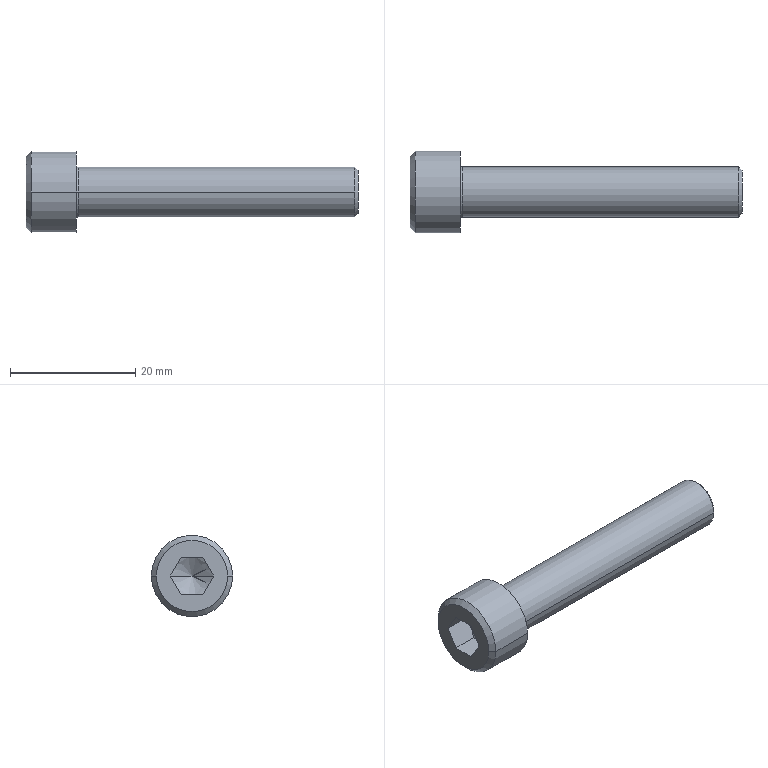Part | Creo | 1 solid | 23 faces | box 53 x 13 x 13 mm | volume 3160 mm3 | plane 9 | cone 6 | cylinder 4 | torus 4 | commonest cylinder face diameters 8 x2 13 x2
STEP:
#1=CARTESIAN_POINT('',(-309.5,39.031,5.));
#2=VERTEX_POINT('',#1);
#3=CARTESIAN_POINT('',(-309.5,40.763,8.));
#4=VERTEX_POINT('',#3);
#5=CARTESIAN_POINT('',(-309.5,39.031,5.));
#6=CARTESIAN_POINT('',(-309.471,39.082,5.088));
#7=CARTESIAN_POINT('',(-309.417,39.182,5.261));
#8=CARTESIAN_POINT('',(-309.351,39.326,5.511));
#9=CARTESIAN_POINT('',(-309.299,39.468,5.757));
#10=CARTESIAN_POINT('',(-309.261,39.61,6.002));
#11=CARTESIAN_POINT('',(-309.237,39.753,6.25));
#12=CARTESIAN_POINT('',(-309.229,39.897,6.5));
#13=CARTESIAN_POINT('',(-309.237,40.041,6.75));
#14=CARTESIAN_POINT('',(-309.261,40.185,6.998));
#15=CARTESIAN_POINT('',(-309.299,40.326,7.243));
#16=CARTESIAN_POINT('',(-309.351,40.468,7.489));
#17=CARTESIAN_POINT('',(-309.417,40.613,7.739));
#18=CARTESIAN_POINT('',(-309.471,40.713,7.912));
#19=CARTESIAN_POINT('',(-309.5,40.763,8.));
#20=B_SPLINE_CURVE_WITH_KNOTS('',3,(#5,#6,#7,#8,#9,#10,#11,#12,#13,#14,#15,#16,#17,#18,#19),.UNSPECIFIED.,.F.,.F.,(4,1,1,1,1,1,1,1,1,1,1,1,4),(0.,0.08333,0.1667,0.25,0.3333,0.4167,0.5,0.5833,0.6667,0.75,0.8333,0.9167,1.),.UNSPECIFIED.);
#21=EDGE_CURVE('',#2,#4,#20,.T.);
#22=ORIENTED_EDGE('',*,*,#21,.F.);
#23=CARTESIAN_POINT('',(-307.5,42.495,5.));
#24=VERTEX_POINT('',#23);
#25=CARTESIAN_POINT('',(-307.5,42.495,5.));
#26=DIRECTION('',(-0.5,-0.866,0.));
#27=VECTOR('',#26,4.);
#28=LINE('',#25,#27);
#29=EDGE_CURVE('',#24,#2,#28,.T.);
#30=ORIENTED_EDGE('',*,*,#29,.F.);
#31=CARTESIAN_POINT('',(-309.5,45.959,5.));
#32=VERTEX_POINT('',#31);
#33=CARTESIAN_POINT('',(-307.5,42.495,5.));
#34=DIRECTION('',(-0.5,0.866,0.));
#35=VECTOR('',#34,4.);
#36=LINE('',#33,#35);
#37=EDGE_CURVE('',#24,#32,#36,.T.);
#38=ORIENTED_EDGE('',*,*,#37,.T.);
#39=CARTESIAN_POINT('',(-309.5,44.227,8.));
#40=VERTEX_POINT('',#39);
#41=CARTESIAN_POINT('',(-309.5,44.227,8.));
#42=CARTESIAN_POINT('',(-309.471,44.278,7.912));
#43=CARTESIAN_POINT('',(-309.417,44.378,7.739));
#44=CARTESIAN_POINT('',(-309.351,44.522,7.489));
#45=CARTESIAN_POINT('',(-309.299,44.664,7.243));
#46=CARTESIAN_POINT('',(-309.261,44.806,6.998));
#47=CARTESIAN_POINT('',(-309.237,44.949,6.75));
#48=CARTESIAN_POINT('',(-309.229,45.093,6.5));
#49=CARTESIAN_POINT('',(-309.237,45.238,6.25));
#50=CARTESIAN_POINT('',(-309.261,45.381,6.002));
#51=CARTESIAN_POINT('',(-309.299,45.522,5.757));
#52=CARTESIAN_POINT('',(-309.351,45.664,5.511));
#53=CARTESIAN_POINT('',(-309.417,45.809,5.261));
#54=CARTESIAN_POINT('',(-309.471,45.909,5.088));
#55=CARTESIAN_POINT('',(-309.5,45.959,5.));
#56=B_SPLINE_CURVE_WITH_KNOTS('',3,(#41,#42,#43,#44,#45,#46,#47,#48,#49,#50,#51,#52,#53,#54,#55),.UNSPECIFIED.,.F.,.F.,(4,1,1,1,1,1,1,1,1,1,1,1,4),(0.,0.08333,0.1667,0.25,0.3333,0.4167,0.5,0.5833,0.6667,0.75,0.8333,0.9167,1.),.UNSPECIFIED.);
#57=EDGE_CURVE('',#40,#32,#56,.T.);
#58=ORIENTED_EDGE('',*,*,#57,.F.);
#59=CARTESIAN_POINT('',(-309.5,40.763,8.));
#60=CARTESIAN_POINT('',(-309.471,40.865,8.));
#61=CARTESIAN_POINT('',(-309.417,41.064,8.));
#62=CARTESIAN_POINT('',(-309.351,41.353,8.));
#63=CARTESIAN_POINT('',(-309.299,41.636,8.));
#64=CARTESIAN_POINT('',(-309.261,41.919,8.));
#65=CARTESIAN_POINT('',(-309.237,42.206,8.));
#66=CARTESIAN_POINT('',(-309.229,42.495,8.));
#67=CARTESIAN_POINT('',(-309.237,42.784,8.));
#68=CARTESIAN_POINT('',(-309.261,43.072,8.));
#69=CARTESIAN_POINT('',(-309.299,43.354,8.));
#70=CARTESIAN_POINT('',(-309.351,43.638,8.));
#71=CARTESIAN_POINT('',(-309.417,43.926,8.));
#72=CARTESIAN_POINT('',(-309.471,44.126,8.));
#73=CARTESIAN_POINT('',(-309.5,44.227,8.));
#74=B_SPLINE_CURVE_WITH_KNOTS('',3,(#59,#60,#61,#62,#63,#64,#65,#66,#67,#68,#69,#70,#71,#72,#73),.UNSPECIFIED.,.F.,.F.,(4,1,1,1,1,1,1,1,1,1,1,1,4),(0.,0.08333,0.1667,0.25,0.3333,0.4167,0.5,0.5833,0.6667,0.75,0.8333,0.9167,1.),.UNSPECIFIED.);
#75=EDGE_CURVE('',#4,#40,#74,.T.);
#76=ORIENTED_EDGE('',*,*,#75,.F.);
#77=EDGE_LOOP('',(#22,#30,#38,#58,#76));
#78=FACE_OUTER_BOUND('',#77,.F.);
#79=CARTESIAN_POINT('',(-308.52,42.495,5.));
#80=DIRECTION('',(-1.,0.,0.));
#81=DIRECTION('',(0.,-1.,0.));
#82=AXIS2_PLACEMENT_3D('',#79,#80,#81);
#83=CONICAL_SURFACE('',#82,1.767,60.);
#84=ADVANCED_FACE('',(#78),#83,.F.);
#85=CARTESIAN_POINT('',(-313.5,40.763,8.));
#86=VERTEX_POINT('',#85);
#87=CARTESIAN_POINT('',(-313.5,39.031,5.));
#88=VERTEX_POINT('',#87);
#89=CARTESIAN_POINT('',(-313.5,40.763,8.));
#90=DIRECTION('',(0.,-0.5,-0.866));
#91=VECTOR('',#90,3.464);
#92=LINE('',#89,#91);
#93=EDGE_CURVE('',#86,#88,#92,.T.);
#94=ORIENTED_EDGE('',*,*,#93,.T.);
#95=CARTESIAN_POINT('',(-313.5,39.031,5.));
#96=DIRECTION('',(1.,0.,0.));
#97=VECTOR('',#96,4.);
#98=LINE('',#95,#97);
#99=EDGE_CURVE('',#88,#2,#98,.T.);
#100=ORIENTED_EDGE('',*,*,#99,.T.);
#101=ORIENTED_EDGE('',*,*,#21,.T.);
#102=CARTESIAN_POINT('',(-313.5,40.763,8.));
#103=DIRECTION('',(1.,0.,0.));
#104=VECTOR('',#103,4.);
#105=LINE('',#102,#104);
#106=EDGE_CURVE('',#86,#4,#105,.T.);
#107=ORIENTED_EDGE('',*,*,#106,.F.);
#108=EDGE_LOOP('',(#94,#100,#101,#107));
#109=FACE_OUTER_BOUND('',#108,.F.);
#110=CARTESIAN_POINT('',(-309.5,40.763,8.));
#111=DIRECTION('',(0.,0.866,-0.5));
#112=DIRECTION('',(0.,-0.5,-0.866));
#113=AXIS2_PLACEMENT_3D('',#110,#111,#112);
#114=PLANE('',#113);
#115=ADVANCED_FACE('',(#109),#114,.T.);
#116=CARTESIAN_POINT('',(-313.5,36.795,5.));
#117=VERTEX_POINT('',#116);
#118=CARTESIAN_POINT('',(-313.5,48.195,5.));
#119=VERTEX_POINT('',#118);
#120=CARTESIAN_POINT('',(-313.5,42.495,5.));
#121=DIRECTION('',(-1.,0.,0.));
#122=DIRECTION('',(0.,-1.,0.));
#123=AXIS2_PLACEMENT_3D('',#120,#121,#122);
#124=CIRCLE('',#123,5.7);
#125=EDGE_CURVE('',#117,#119,#124,.T.);
#126=ORIENTED_EDGE('',*,*,#125,.F.);
#127=CARTESIAN_POINT('',(-313.5,42.495,5.));
#128=DIRECTION('',(-1.,0.,0.));
#129=DIRECTION('',(0.,1.,0.));
#130=AXIS2_PLACEMENT_3D('',#127,#128,#129);
#131=CIRCLE('',#130,5.7);
#132=EDGE_CURVE('',#119,#117,#131,.T.);
#133=ORIENTED_EDGE('',*,*,#132,.F.);
#134=EDGE_LOOP('',(#126,#133));
#135=FACE_OUTER_BOUND('',#134,.F.);
#136=CARTESIAN_POINT('',(-313.5,40.763,2.));
#137=VERTEX_POINT('',#136);
#138=CARTESIAN_POINT('',(-313.5,39.031,5.));
#139=DIRECTION('',(0.,0.5,-0.866));
#140=VECTOR('',#139,3.464);
#141=LINE('',#138,#140);
#142=EDGE_CURVE('',#88,#137,#141,.T.);
#143=ORIENTED_EDGE('',*,*,#142,.F.);
#144=ORIENTED_EDGE('',*,*,#93,.F.);
#145=CARTESIAN_POINT('',(-313.5,44.227,8.));
#146=VERTEX_POINT('',#145);
#147=CARTESIAN_POINT('',(-313.5,40.763,8.));
#148=DIRECTION('',(0.,1.,0.));
#149=VECTOR('',#148,3.464);
#150=LINE('',#147,#149);
#151=EDGE_CURVE('',#86,#146,#150,.T.);
#152=ORIENTED_EDGE('',*,*,#151,.T.);
#153=CARTESIAN_POINT('',(-313.5,45.959,5.));
#154=VERTEX_POINT('',#153);
#155=CARTESIAN_POINT('',(-313.5,45.959,5.));
#156=DIRECTION('',(0.,-0.5,0.866));
#157=VECTOR('',#156,3.464);
#158=LINE('',#155,#157);
#159=EDGE_CURVE('',#154,#146,#158,.T.);
#160=ORIENTED_EDGE('',*,*,#159,.F.);
#161=CARTESIAN_POINT('',(-313.5,44.227,2.));
#162=VERTEX_POINT('',#161);
#163=CARTESIAN_POINT('',(-313.5,44.227,2.));
#164=DIRECTION('',(0.,0.5,0.866));
#165=VECTOR('',#164,3.464);
#166=LINE('',#163,#165);
#167=EDGE_CURVE('',#162,#154,#166,.T.);
#168=ORIENTED_EDGE('',*,*,#167,.F.);
#169=CARTESIAN_POINT('',(-313.5,44.227,2.));
#170=DIRECTION('',(0.,-1.,0.));
#171=VECTOR('',#170,3.464);
#172=LINE('',#169,#171);
#173=EDGE_CURVE('',#162,#137,#172,.T.);
#174=ORIENTED_EDGE('',*,*,#173,.T.);
#175=EDGE_LOOP('',(#143,#144,#152,#160,#168,#174));
#176=FACE_BOUND('',#175,.F.);
#177=CARTESIAN_POINT('',(-313.5,42.495,5.));
#178=DIRECTION('',(-1.,0.,0.));
#179=DIRECTION('',(0.,-1.,0.));
#180=AXIS2_PLACEMENT_3D('',#177,#178,#179);
#181=PLANE('',#180);
#182=ADVANCED_FACE('',(#135,#176),#181,.T.);
#183=CARTESIAN_POINT('',(-312.7,35.995,5.));
#184=VERTEX_POINT('',#183);
#185=CARTESIAN_POINT('',(-312.7,48.995,5.));
#186=VERTEX_POINT('',#185);
#187=CARTESIAN_POINT('',(-312.7,42.495,5.));
#188=DIRECTION('',(-1.,0.,0.));
#189=DIRECTION('',(0.,-1.,0.));
#190=AXIS2_PLACEMENT_3D('',#187,#188,#189);
#191=CIRCLE('',#190,6.5);
#192=EDGE_CURVE('',#184,#186,#191,.T.);
#193=ORIENTED_EDGE('',*,*,#192,.F.);
#194=CARTESIAN_POINT('',(-313.5,36.795,5.));
#195=DIRECTION('',(0.7071,-0.7071,0.));
#196=VECTOR('',#195,1.131);
#197=LINE('',#194,#196);
#198=EDGE_CURVE('',#117,#184,#197,.T.);
#199=ORIENTED_EDGE('',*,*,#198,.F.);
#200=ORIENTED_EDGE('',*,*,#125,.T.);
#201=CARTESIAN_POINT('',(-313.5,48.195,5.));
#202=DIRECTION('',(0.7071,0.7071,0.));
#203=VECTOR('',#202,1.131);
#204=LINE('',#201,#203);
#205=EDGE_CURVE('',#119,#186,#204,.T.);
#206=ORIENTED_EDGE('',*,*,#205,.T.);
#207=EDGE_LOOP('',(#193,#199,#200,#206));
#208=FACE_OUTER_BOUND('',#207,.F.);
#209=CARTESIAN_POINT('',(-313.1,42.495,5.));
#210=DIRECTION('',(1.,0.,0.));
#211=DIRECTION('',(0.,1.,0.));
#212=AXIS2_PLACEMENT_3D('',#209,#210,#211);
#213=CONICAL_SURFACE('',#212,6.1,45.);
#214=ADVANCED_FACE('',(#208),#213,.T.);
#215=ORIENTED_EDGE('',*,*,#192,.T.);
#216=CARTESIAN_POINT('',(-305.5,48.995,5.));
#217=VERTEX_POINT('',#216);
#218=CARTESIAN_POINT('',(-305.5,48.995,5.));
#219=DIRECTION('',(-1.,0.,0.));
#220=VECTOR('',#219,7.2);
#221=LINE('',#218,#220);
#222=EDGE_CURVE('',#217,#186,#221,.T.);
#223=ORIENTED_EDGE('',*,*,#222,.F.);
#224=CARTESIAN_POINT('',(-305.5,35.995,5.));
#225=VERTEX_POINT('',#224);
#226=CARTESIAN_POINT('',(-305.5,42.495,5.));
#227=DIRECTION('',(1.,0.,0.));
#228=DIRECTION('',(0.,1.,0.));
#229=AXIS2_PLACEMENT_3D('',#226,#227,#228);
#230=CIRCLE('',#229,6.5);
#231=EDGE_CURVE('',#217,#225,#230,.T.);
#232=ORIENTED_EDGE('',*,*,#231,.T.);
#233=CARTESIAN_POINT('',(-305.5,35.995,5.));
#234=DIRECTION('',(-1.,0.,0.));
#235=VECTOR('',#234,7.2);
#236=LINE('',#233,#235);
#237=EDGE_CURVE('',#225,#184,#236,.T.);
#238=ORIENTED_EDGE('',*,*,#237,.T.);
#239=EDGE_LOOP('',(#215,#223,#232,#238));
#240=FACE_OUTER_BOUND('',#239,.F.);
#241=CARTESIAN_POINT('',(-305.5,42.495,5.));
#242=DIRECTION('',(-1.,0.,0.));
#243=DIRECTION('',(0.,-1.,0.));
#244=AXIS2_PLACEMENT_3D('',#241,#242,#243);
#245=CYLINDRICAL_SURFACE('',#244,6.5);
#246=ADVANCED_FACE('',(#240),#245,.T.);
#247=CARTESIAN_POINT('',(-312.7,42.495,5.));
#248=DIRECTION('',(-1.,0.,0.));
#249=DIRECTION('',(0.,1.,0.));
#250=AXIS2_PLACEMENT_3D('',#247,#248,#249);
#251=CIRCLE('',#250,6.5);
#252=EDGE_CURVE('',#186,#184,#251,.T.);
#253=ORIENTED_EDGE('',*,*,#252,.T.);
#254=ORIENTED_EDGE('',*,*,#237,.F.);
#255=CARTESIAN_POINT('',(-305.5,42.495,5.));
#256=DIRECTION('',(1.,0.,0.));
#257=DIRECTION('',(0.,-1.,0.));
#258=AXIS2_PLACEMENT_3D('',#255,#256,#257);
#259=CIRCLE('',#258,6.5);
#260=EDGE_CURVE('',#225,#217,#259,.T.);
#261=ORIENTED_EDGE('',*,*,#260,.T.);
#262=ORIENTED_EDGE('',*,*,#222,.T.);
#263=EDGE_LOOP('',(#253,#254,#261,#262));
#264=FACE_OUTER_BOUND('',#263,.F.);
#265=CARTESIAN_POINT('',(-305.5,42.495,5.));
#266=DIRECTION('',(-1.,0.,0.));
#267=DIRECTION('',(0.,-1.,0.));
#268=AXIS2_PLACEMENT_3D('',#265,#266,#267);
#269=CYLINDRICAL_SURFACE('',#268,6.5);
#270=ADVANCED_FACE('',(#264),#269,.T.);
#271=ORIENTED_EDGE('',*,*,#252,.F.);
#272=ORIENTED_EDGE('',*,*,#205,.F.);
#273=ORIENTED_EDGE('',*,*,#132,.T.);
#274=ORIENTED_EDGE('',*,*,#198,.T.);
#275=EDGE_LOOP('',(#271,#272,#273,#274));
#276=FACE_OUTER_BOUND('',#275,.F.);
#277=CARTESIAN_POINT('',(-313.1,42.495,5.));
#278=DIRECTION('',(1.,0.,0.));
#279=DIRECTION('',(0.,1.,0.));
#280=AXIS2_PLACEMENT_3D('',#277,#278,#279);
#281=CONICAL_SURFACE('',#280,6.1,45.);
#282=ADVANCED_FACE('',(#276),#281,.T.);
#283=ORIENTED_EDGE('',*,*,#260,.F.);
#284=ORIENTED_EDGE('',*,*,#231,.F.);
#285=EDGE_LOOP('',(#283,#284));
#286=FACE_OUTER_BOUND('',#285,.F.);
#287=CARTESIAN_POINT('',(-305.5,38.095,5.));
#288=VERTEX_POINT('',#287);
#289=CARTESIAN_POINT('',(-305.5,46.895,5.));
#290=VERTEX_POINT('',#289);
#291=CARTESIAN_POINT('',(-305.5,42.495,5.));
#292=DIRECTION('',(-1.,0.,0.));
#293=DIRECTION('',(0.,-1.,0.));
#294=AXIS2_PLACEMENT_3D('',#291,#292,#293);
#295=CIRCLE('',#294,4.4);
#296=EDGE_CURVE('',#288,#290,#295,.T.);
#297=ORIENTED_EDGE('',*,*,#296,.F.);
#298=CARTESIAN_POINT('',(-305.5,42.495,5.));
#299=DIRECTION('',(-1.,0.,0.));
#300=DIRECTION('',(0.,1.,0.));
#301=AXIS2_PLACEMENT_3D('',#298,#299,#300);
#302=CIRCLE('',#301,4.4);
#303=EDGE_CURVE('',#290,#288,#302,.T.);
#304=ORIENTED_EDGE('',*,*,#303,.F.);
#305=EDGE_LOOP('',(#297,#304));
#306=FACE_BOUND('',#305,.F.);
#307=CARTESIAN_POINT('',(-305.5,42.495,5.));
#308=DIRECTION('',(-1.,0.,0.));
#309=DIRECTION('',(0.,-1.,0.));
#310=AXIS2_PLACEMENT_3D('',#307,#308,#309);
#311=PLANE('',#310);
#312=ADVANCED_FACE('',(#286,#306),#311,.F.);
#313=ORIENTED_EDGE('',*,*,#296,.T.);
#314=CARTESIAN_POINT('',(-305.383,46.612,5.));
#315=VERTEX_POINT('',#314);
#316=CARTESIAN_POINT('',(-305.1,46.895,5.));
#317=DIRECTION('',(0.,0.,1.));
#318=DIRECTION('',(-1.,0.,0.));
#319=AXIS2_PLACEMENT_3D('',#316,#317,#318);
#320=CIRCLE('',#319,0.4);
#321=EDGE_CURVE('',#290,#315,#320,.T.);
#322=ORIENTED_EDGE('',*,*,#321,.T.);
#323=CARTESIAN_POINT('',(-305.383,38.378,5.));
#324=VERTEX_POINT('',#323);
#325=CARTESIAN_POINT('',(-305.383,42.495,5.));
#326=DIRECTION('',(-1.,0.,0.));
#327=DIRECTION('',(0.,-1.,0.));
#328=AXIS2_PLACEMENT_3D('',#325,#326,#327);
#329=CIRCLE('',#328,4.117);
#330=EDGE_CURVE('',#324,#315,#329,.T.);
#331=ORIENTED_EDGE('',*,*,#330,.F.);
#332=CARTESIAN_POINT('',(-305.1,38.095,5.));
#333=DIRECTION('',(0.,0.,-1.));
#334=DIRECTION('',(-1.,0.,0.));
#335=AXIS2_PLACEMENT_3D('',#332,#333,#334);
#336=CIRCLE('',#335,0.4);
#337=EDGE_CURVE('',#288,#324,#336,.T.);
#338=ORIENTED_EDGE('',*,*,#337,.F.);
#339=EDGE_LOOP('',(#313,#322,#331,#338));
#340=FACE_OUTER_BOUND('',#339,.F.);
#341=CARTESIAN_POINT('',(-305.1,42.495,5.));
#342=DIRECTION('',(-1.,0.,0.));
#343=DIRECTION('',(0.,-1.,0.));
#344=AXIS2_PLACEMENT_3D('',#341,#342,#343);
#345=TOROIDAL_SURFACE('',#344,4.4,0.4);
#346=ADVANCED_FACE('',(#340),#345,.F.);
#347=ORIENTED_EDGE('',*,*,#303,.T.);
#348=ORIENTED_EDGE('',*,*,#337,.T.);
#349=CARTESIAN_POINT('',(-305.383,42.495,5.));
#350=DIRECTION('',(-1.,0.,0.));
#351=DIRECTION('',(0.,1.,0.));
#352=AXIS2_PLACEMENT_3D('',#349,#350,#351);
#353=CIRCLE('',#352,4.117);
#354=EDGE_CURVE('',#315,#324,#353,.T.);
#355=ORIENTED_EDGE('',*,*,#354,.F.);
#356=ORIENTED_EDGE('',*,*,#321,.F.);
#357=EDGE_LOOP('',(#347,#348,#355,#356));
#358=FACE_OUTER_BOUND('',#357,.F.);
#359=CARTESIAN_POINT('',(-305.1,42.495,5.));
#360=DIRECTION('',(-1.,0.,0.));
#361=DIRECTION('',(0.,-1.,0.));
#362=AXIS2_PLACEMENT_3D('',#359,#360,#361);
#363=TOROIDAL_SURFACE('',#362,4.4,0.4);
#364=ADVANCED_FACE('',(#358),#363,.F.);
#365=CARTESIAN_POINT('',(-305.1,46.495,5.));
#366=VERTEX_POINT('',#365);
#367=CARTESIAN_POINT('',(-305.1,38.495,5.));
#368=VERTEX_POINT('',#367);
#369=CARTESIAN_POINT('',(-305.1,42.495,5.));
#370=DIRECTION('',(-1.,0.,0.));
#371=DIRECTION('',(0.,1.,0.));
#372=AXIS2_PLACEMENT_3D('',#369,#370,#371);
#373=CIRCLE('',#372,4.);
#374=EDGE_CURVE('',#366,#368,#373,.T.);
#375=ORIENTED_EDGE('',*,*,#374,.F.);
#376=CARTESIAN_POINT('',(-305.1,46.895,5.));
#377=DIRECTION('',(0.,0.,1.));
#378=DIRECTION('',(-0.7071,-0.7071,0.));
#379=AXIS2_PLACEMENT_3D('',#376,#377,#378);
#380=CIRCLE('',#379,0.4);
#381=EDGE_CURVE('',#315,#366,#380,.T.);
#382=ORIENTED_EDGE('',*,*,#381,.F.);
#383=ORIENTED_EDGE('',*,*,#354,.T.);
#384=CARTESIAN_POINT('',(-305.1,38.095,5.));
#385=DIRECTION('',(0.,0.,-1.));
#386=DIRECTION('',(-0.7071,0.7071,0.));
#387=AXIS2_PLACEMENT_3D('',#384,#385,#386);
#388=CIRCLE('',#387,0.4);
#389=EDGE_CURVE('',#324,#368,#388,.T.);
#390=ORIENTED_EDGE('',*,*,#389,.T.);
#391=EDGE_LOOP('',(#375,#382,#383,#390));
#392=FACE_OUTER_BOUND('',#391,.F.);
#393=CARTESIAN_POINT('',(-305.1,42.495,5.));
#394=DIRECTION('',(-1.,0.,0.));
#395=DIRECTION('',(0.,-1.,0.));
#396=AXIS2_PLACEMENT_3D('',#393,#394,#395);
#397=TOROIDAL_SURFACE('',#396,4.4,0.4);
#398=ADVANCED_FACE('',(#392),#397,.F.);
#399=CARTESIAN_POINT('',(-261.,38.495,5.));
#400=VERTEX_POINT('',#399);
#401=CARTESIAN_POINT('',(-261.,46.495,5.));
#402=VERTEX_POINT('',#401);
#403=CARTESIAN_POINT('',(-261.,42.495,5.));
#404=DIRECTION('',(1.,0.,0.));
#405=DIRECTION('',(0.,-1.,0.));
#406=AXIS2_PLACEMENT_3D('',#403,#404,#405);
#407=CIRCLE('',#406,4.);
#408=EDGE_CURVE('',#400,#402,#407,.T.);
#409=ORIENTED_EDGE('',*,*,#408,.T.);
#410=CARTESIAN_POINT('',(-261.,46.495,5.));
#411=DIRECTION('',(-1.,0.,0.));
#412=VECTOR('',#411,44.1);
#413=LINE('',#410,#412);
#414=EDGE_CURVE('',#402,#366,#413,.T.);
#415=ORIENTED_EDGE('',*,*,#414,.T.);
#416=ORIENTED_EDGE('',*,*,#374,.T.);
#417=CARTESIAN_POINT('',(-261.,38.495,5.));
#418=DIRECTION('',(-1.,0.,0.));
#419=VECTOR('',#418,44.1);
#420=LINE('',#417,#419);
#421=EDGE_CURVE('',#400,#368,#420,.T.);
#422=ORIENTED_EDGE('',*,*,#421,.F.);
#423=EDGE_LOOP('',(#409,#415,#416,#422));
#424=FACE_OUTER_BOUND('',#423,.F.);
#425=CARTESIAN_POINT('',(-260.5,42.495,5.));
#426=DIRECTION('',(-1.,0.,0.));
#427=DIRECTION('',(0.,-1.,0.));
#428=AXIS2_PLACEMENT_3D('',#425,#426,#427);
#429=CYLINDRICAL_SURFACE('',#428,4.);
#430=ADVANCED_FACE('',(#424),#429,.T.);
#431=CARTESIAN_POINT('',(-260.5,38.995,5.));
#432=VERTEX_POINT('',#431);
#433=CARTESIAN_POINT('',(-260.5,45.995,5.));
#434=VERTEX_POINT('',#433);
#435=CARTESIAN_POINT('',(-260.5,42.495,5.));
#436=DIRECTION('',(1.,0.,0.));
#437=DIRECTION('',(0.,-1.,0.));
#438=AXIS2_PLACEMENT_3D('',#435,#436,#437);
#439=CIRCLE('',#438,3.5);
#440=EDGE_CURVE('',#432,#434,#439,.T.);
#441=ORIENTED_EDGE('',*,*,#440,.T.);
#442=CARTESIAN_POINT('',(-260.5,45.995,5.));
#443=DIRECTION('',(-0.7071,0.7071,0.));
#444=VECTOR('',#443,0.7071);
#445=LINE('',#442,#444);
#446=EDGE_CURVE('',#434,#402,#445,.T.);
#447=ORIENTED_EDGE('',*,*,#446,.T.);
#448=ORIENTED_EDGE('',*,*,#408,.F.);
#449=CARTESIAN_POINT('',(-260.5,38.995,5.));
#450=DIRECTION('',(-0.7071,-0.7071,0.));
#451=VECTOR('',#450,0.7071);
#452=LINE('',#449,#451);
#453=EDGE_CURVE('',#432,#400,#452,.T.);
#454=ORIENTED_EDGE('',*,*,#453,.F.);
#455=EDGE_LOOP('',(#441,#447,#448,#454));
#456=FACE_OUTER_BOUND('',#455,.F.);
#457=CARTESIAN_POINT('',(-260.75,42.495,5.));
#458=DIRECTION('',(-1.,0.,0.));
#459=DIRECTION('',(0.,-1.,0.));
#460=AXIS2_PLACEMENT_3D('',#457,#458,#459);
#461=CONICAL_SURFACE('',#460,3.75,45.);
#462=ADVANCED_FACE('',(#456),#461,.T.);
#463=ORIENTED_EDGE('',*,*,#440,.F.);
#464=CARTESIAN_POINT('',(-260.5,42.495,5.));
#465=DIRECTION('',(1.,0.,0.));
#466=DIRECTION('',(0.,1.,0.));
#467=AXIS2_PLACEMENT_3D('',#464,#465,#466);
#468=CIRCLE('',#467,3.5);
#469=EDGE_CURVE('',#434,#432,#468,.T.);
#470=ORIENTED_EDGE('',*,*,#469,.F.);
#471=EDGE_LOOP('',(#463,#470));
#472=FACE_OUTER_BOUND('',#471,.F.);
#473=CARTESIAN_POINT('',(-260.5,42.495,5.));
#474=DIRECTION('',(-1.,0.,0.));
#475=DIRECTION('',(0.,-1.,0.));
#476=AXIS2_PLACEMENT_3D('',#473,#474,#475);
#477=PLANE('',#476);
#478=ADVANCED_FACE('',(#472),#477,.F.);
#479=ORIENTED_EDGE('',*,*,#469,.T.);
#480=ORIENTED_EDGE('',*,*,#453,.T.);
#481=CARTESIAN_POINT('',(-261.,42.495,5.));
#482=DIRECTION('',(1.,0.,0.));
#483=DIRECTION('',(0.,1.,0.));
#484=AXIS2_PLACEMENT_3D('',#481,#482,#483);
#485=CIRCLE('',#484,4.);
#486=EDGE_CURVE('',#402,#400,#485,.T.);
#487=ORIENTED_EDGE('',*,*,#486,.F.);
#488=ORIENTED_EDGE('',*,*,#446,.F.);
#489=EDGE_LOOP('',(#479,#480,#487,#488));
#490=FACE_OUTER_BOUND('',#489,.F.);
#491=CARTESIAN_POINT('',(-260.75,42.495,5.));
#492=DIRECTION('',(-1.,0.,0.));
#493=DIRECTION('',(0.,-1.,0.));
#494=AXIS2_PLACEMENT_3D('',#491,#492,#493);
#495=CONICAL_SURFACE('',#494,3.75,45.);
#496=ADVANCED_FACE('',(#490),#495,.T.);
#497=ORIENTED_EDGE('',*,*,#486,.T.);
#498=ORIENTED_EDGE('',*,*,#421,.T.);
#499=CARTESIAN_POINT('',(-305.1,42.495,5.));
#500=DIRECTION('',(-1.,0.,0.));
#501=DIRECTION('',(0.,-1.,0.));
#502=AXIS2_PLACEMENT_3D('',#499,#500,#501);
#503=CIRCLE('',#502,4.);
#504=EDGE_CURVE('',#368,#366,#503,.T.);
#505=ORIENTED_EDGE('',*,*,#504,.T.);
#506=ORIENTED_EDGE('',*,*,#414,.F.);
#507=EDGE_LOOP('',(#497,#498,#505,#506));
#508=FACE_OUTER_BOUND('',#507,.F.);
#509=CARTESIAN_POINT('',(-260.5,42.495,5.));
#510=DIRECTION('',(-1.,0.,0.));
#511=DIRECTION('',(0.,-1.,0.));
#512=AXIS2_PLACEMENT_3D('',#509,#510,#511);
#513=CYLINDRICAL_SURFACE('',#512,4.);
#514=ADVANCED_FACE('',(#508),#513,.T.);
#515=ORIENTED_EDGE('',*,*,#504,.F.);
#516=ORIENTED_EDGE('',*,*,#389,.F.);
#517=ORIENTED_EDGE('',*,*,#330,.T.);
#518=ORIENTED_EDGE('',*,*,#381,.T.);
#519=EDGE_LOOP('',(#515,#516,#517,#518));
#520=FACE_OUTER_BOUND('',#519,.F.);
#521=CARTESIAN_POINT('',(-305.1,42.495,5.));
#522=DIRECTION('',(-1.,0.,0.));
#523=DIRECTION('',(0.,-1.,0.));
#524=AXIS2_PLACEMENT_3D('',#521,#522,#523);
#525=TOROIDAL_SURFACE('',#524,4.4,0.4);
#526=ADVANCED_FACE('',(#520),#525,.F.);
#527=ORIENTED_EDGE('',*,*,#142,.T.);
#528=CARTESIAN_POINT('',(-309.5,40.763,2.));
#529=VERTEX_POINT('',#528);
#530=CARTESIAN_POINT('',(-313.5,40.763,2.));
#531=DIRECTION('',(1.,0.,0.));
#532=VECTOR('',#531,4.);
#533=LINE('',#530,#532);
#534=EDGE_CURVE('',#137,#529,#533,.T.);
#535=ORIENTED_EDGE('',*,*,#534,.T.);
#536=CARTESIAN_POINT('',(-309.5,40.763,2.));
#537=CARTESIAN_POINT('',(-309.471,40.713,2.088));
#538=CARTESIAN_POINT('',(-309.417,40.613,2.261));
#539=CARTESIAN_POINT('',(-309.351,40.468,2.511));
#540=CARTESIAN_POINT('',(-309.299,40.326,2.757));
#541=CARTESIAN_POINT('',(-309.261,40.185,3.002));
#542=CARTESIAN_POINT('',(-309.237,40.041,3.25));
#543=CARTESIAN_POINT('',(-309.229,39.897,3.5));
#544=CARTESIAN_POINT('',(-309.237,39.753,3.75));
#545=CARTESIAN_POINT('',(-309.261,39.61,3.998));
#546=CARTESIAN_POINT('',(-309.299,39.468,4.243));
#547=CARTESIAN_POINT('',(-309.351,39.326,4.489));
#548=CARTESIAN_POINT('',(-309.417,39.182,4.739));
#549=CARTESIAN_POINT('',(-309.471,39.082,4.912));
#550=CARTESIAN_POINT('',(-309.5,39.031,5.));
#551=B_SPLINE_CURVE_WITH_KNOTS('',3,(#536,#537,#538,#539,#540,#541,#542,#543,#544,#545,#546,#547,#548,#549,#550),.UNSPECIFIED.,.F.,.F.,(4,1,1,1,1,1,1,1,1,1,1,1,4),(0.,0.08333,0.1667,0.25,0.3333,0.4167,0.5,0.5833,0.6667,0.75,0.8333,0.9167,1.),.UNSPECIFIED.);
#552=EDGE_CURVE('',#529,#2,#551,.T.);
#553=ORIENTED_EDGE('',*,*,#552,.T.);
#554=ORIENTED_EDGE('',*,*,#99,.F.);
#555=EDGE_LOOP('',(#527,#535,#553,#554));
#556=FACE_OUTER_BOUND('',#555,.F.);
#557=CARTESIAN_POINT('',(-309.5,39.031,5.));
#558=DIRECTION('',(0.,0.866,0.5));
#559=DIRECTION('',(0.,0.5,-0.866));
#560=AXIS2_PLACEMENT_3D('',#557,#558,#559);
#561=PLANE('',#560);
#562=ADVANCED_FACE('',(#556),#561,.T.);
#563=ORIENTED_EDGE('',*,*,#173,.F.);
#564=CARTESIAN_POINT('',(-309.5,44.227,2.));
#565=VERTEX_POINT('',#564);
#566=CARTESIAN_POINT('',(-313.5,44.227,2.));
#567=DIRECTION('',(1.,0.,0.));
#568=VECTOR('',#567,4.);
#569=LINE('',#566,#568);
#570=EDGE_CURVE('',#162,#565,#569,.T.);
#571=ORIENTED_EDGE('',*,*,#570,.T.);
#572=CARTESIAN_POINT('',(-309.5,44.227,2.));
#573=CARTESIAN_POINT('',(-309.471,44.126,2.));
#574=CARTESIAN_POINT('',(-309.417,43.926,2.));
#575=CARTESIAN_POINT('',(-309.351,43.638,2.));
#576=CARTESIAN_POINT('',(-309.299,43.354,2.));
#577=CARTESIAN_POINT('',(-309.261,43.072,2.));
#578=CARTESIAN_POINT('',(-309.237,42.784,2.));
#579=CARTESIAN_POINT('',(-309.229,42.495,2.));
#580=CARTESIAN_POINT('',(-309.237,42.206,2.));
#581=CARTESIAN_POINT('',(-309.261,41.919,2.));
#582=CARTESIAN_POINT('',(-309.299,41.636,2.));
#583=CARTESIAN_POINT('',(-309.351,41.353,2.));
#584=CARTESIAN_POINT('',(-309.417,41.064,2.));
#585=CARTESIAN_POINT('',(-309.471,40.865,2.));
#586=CARTESIAN_POINT('',(-309.5,40.763,2.));
#587=B_SPLINE_CURVE_WITH_KNOTS('',3,(#572,#573,#574,#575,#576,#577,#578,#579,#580,#581,#582,#583,#584,#585,#586),.UNSPECIFIED.,.F.,.F.,(4,1,1,1,1,1,1,1,1,1,1,1,4),(0.,0.08333,0.1667,0.25,0.3333,0.4167,0.5,0.5833,0.6667,0.75,0.8333,0.9167,1.),.UNSPECIFIED.);
#588=EDGE_CURVE('',#565,#529,#587,.T.);
#589=ORIENTED_EDGE('',*,*,#588,.T.);
#590=ORIENTED_EDGE('',*,*,#534,.F.);
#591=EDGE_LOOP('',(#563,#571,#589,#590));
#592=FACE_OUTER_BOUND('',#591,.F.);
#593=CARTESIAN_POINT('',(-309.5,40.763,2.));
#594=DIRECTION('',(0.,0.,1.));
#595=DIRECTION('',(-1.,0.,0.));
#596=AXIS2_PLACEMENT_3D('',#593,#594,#595);
#597=PLANE('',#596);
#598=ADVANCED_FACE('',(#592),#597,.T.);
#599=ORIENTED_EDGE('',*,*,#167,.T.);
#600=CARTESIAN_POINT('',(-313.5,45.959,5.));
#601=DIRECTION('',(1.,0.,0.));
#602=VECTOR('',#601,4.);
#603=LINE('',#600,#602);
#604=EDGE_CURVE('',#154,#32,#603,.T.);
#605=ORIENTED_EDGE('',*,*,#604,.T.);
#606=CARTESIAN_POINT('',(-309.5,45.959,5.));
#607=CARTESIAN_POINT('',(-309.471,45.909,4.912));
#608=CARTESIAN_POINT('',(-309.417,45.809,4.739));
#609=CARTESIAN_POINT('',(-309.351,45.664,4.489));
#610=CARTESIAN_POINT('',(-309.299,45.522,4.243));
#611=CARTESIAN_POINT('',(-309.261,45.381,3.998));
#612=CARTESIAN_POINT('',(-309.237,45.238,3.75));
#613=CARTESIAN_POINT('',(-309.229,45.093,3.5));
#614=CARTESIAN_POINT('',(-309.237,44.949,3.25));
#615=CARTESIAN_POINT('',(-309.261,44.806,3.002));
#616=CARTESIAN_POINT('',(-309.299,44.664,2.757));
#617=CARTESIAN_POINT('',(-309.351,44.522,2.511));
#618=CARTESIAN_POINT('',(-309.417,44.378,2.261));
#619=CARTESIAN_POINT('',(-309.471,44.278,2.088));
#620=CARTESIAN_POINT('',(-309.5,44.227,2.));
#621=B_SPLINE_CURVE_WITH_KNOTS('',3,(#606,#607,#608,#609,#610,#611,#612,#613,#614,#615,#616,#617,#618,#619,#620),.UNSPECIFIED.,.F.,.F.,(4,1,1,1,1,1,1,1,1,1,1,1,4),(0.,0.08333,0.1667,0.25,0.3333,0.4167,0.5,0.5833,0.6667,0.75,0.8333,0.9167,1.),.UNSPECIFIED.);
#622=EDGE_CURVE('',#32,#565,#621,.T.);
#623=ORIENTED_EDGE('',*,*,#622,.T.);
#624=ORIENTED_EDGE('',*,*,#570,.F.);
#625=EDGE_LOOP('',(#599,#605,#623,#624));
#626=FACE_OUTER_BOUND('',#625,.F.);
#627=CARTESIAN_POINT('',(-309.5,44.227,2.));
#628=DIRECTION('',(0.,-0.866,0.5));
#629=DIRECTION('',(0.,0.5,0.866));
#630=AXIS2_PLACEMENT_3D('',#627,#628,#629);
#631=PLANE('',#630);
#632=ADVANCED_FACE('',(#626),#631,.T.);
#633=ORIENTED_EDGE('',*,*,#159,.T.);
#634=CARTESIAN_POINT('',(-313.5,44.227,8.));
#635=DIRECTION('',(1.,0.,0.));
#636=VECTOR('',#635,4.);
#637=LINE('',#634,#636);
#638=EDGE_CURVE('',#146,#40,#637,.T.);
#639=ORIENTED_EDGE('',*,*,#638,.T.);
#640=ORIENTED_EDGE('',*,*,#57,.T.);
#641=ORIENTED_EDGE('',*,*,#604,.F.);
#642=EDGE_LOOP('',(#633,#639,#640,#641));
#643=FACE_OUTER_BOUND('',#642,.F.);
#644=CARTESIAN_POINT('',(-309.5,45.959,5.));
#645=DIRECTION('',(0.,-0.866,-0.5));
#646=DIRECTION('',(0.,-0.5,0.866));
#647=AXIS2_PLACEMENT_3D('',#644,#645,#646);
#648=PLANE('',#647);
#649=ADVANCED_FACE('',(#643),#648,.T.);
#650=ORIENTED_EDGE('',*,*,#151,.F.);
#651=ORIENTED_EDGE('',*,*,#106,.T.);
#652=ORIENTED_EDGE('',*,*,#75,.T.);
#653=ORIENTED_EDGE('',*,*,#638,.F.);
#654=EDGE_LOOP('',(#650,#651,#652,#653));
#655=FACE_OUTER_BOUND('',#654,.F.);
#656=CARTESIAN_POINT('',(-309.5,44.227,8.));
#657=DIRECTION('',(0.,0.,-1.));
#658=DIRECTION('',(1.,0.,0.));
#659=AXIS2_PLACEMENT_3D('',#656,#657,#658);
#660=PLANE('',#659);
#661=ADVANCED_FACE('',(#655),#660,.T.);
#662=ORIENTED_EDGE('',*,*,#622,.F.);
#663=ORIENTED_EDGE('',*,*,#37,.F.);
#664=ORIENTED_EDGE('',*,*,#29,.T.);
#665=ORIENTED_EDGE('',*,*,#552,.F.);
#666=ORIENTED_EDGE('',*,*,#588,.F.);
#667=EDGE_LOOP('',(#662,#663,#664,#665,#666));
#668=FACE_OUTER_BOUND('',#667,.F.);
#669=CARTESIAN_POINT('',(-308.52,42.495,5.));
#670=DIRECTION('',(-1.,0.,0.));
#671=DIRECTION('',(0.,-1.,0.));
#672=AXIS2_PLACEMENT_3D('',#669,#670,#671);
#673=CONICAL_SURFACE('',#672,1.767,60.);
#674=ADVANCED_FACE('',(#668),#673,.F.);
#675=CLOSED_SHELL('',(#84,#115,#182,#214,#246,#270,#282,#312,#346,#364,#398,#430,#462,#478,#496,#514,#526,#562,#598,#632,#649,#661,#674));
#676=MANIFOLD_SOLID_BREP('',#675);
#677=(LENGTH_UNIT()NAMED_UNIT(*)SI_UNIT(.MILLI.,.METRE.));
#678=UNCERTAINTY_MEASURE_WITH_UNIT(LENGTH_MEASURE(0.00561),#677,'','');
#679=(NAMED_UNIT(*)PLANE_ANGLE_UNIT()SI_UNIT($,.RADIAN.));
#680=PLANE_ANGLE_MEASURE_WITH_UNIT(PLANE_ANGLE_MEASURE(0.01745),#679);
#681=(CONVERSION_BASED_UNIT('DEGREE',#680)NAMED_UNIT(*)PLANE_ANGLE_UNIT());
#682=(NAMED_UNIT(*)SI_UNIT($,.STERADIAN.)SOLID_ANGLE_UNIT());
#683=(GEOMETRIC_REPRESENTATION_CONTEXT(3)GLOBAL_UNCERTAINTY_ASSIGNED_CONTEXT((#678))GLOBAL_UNIT_ASSIGNED_CONTEXT((#677,#681,#682))REPRESENTATION_CONTEXT('',''));
#684=ADVANCED_BREP_SHAPE_REPRESENTATION('',(#676),#683);